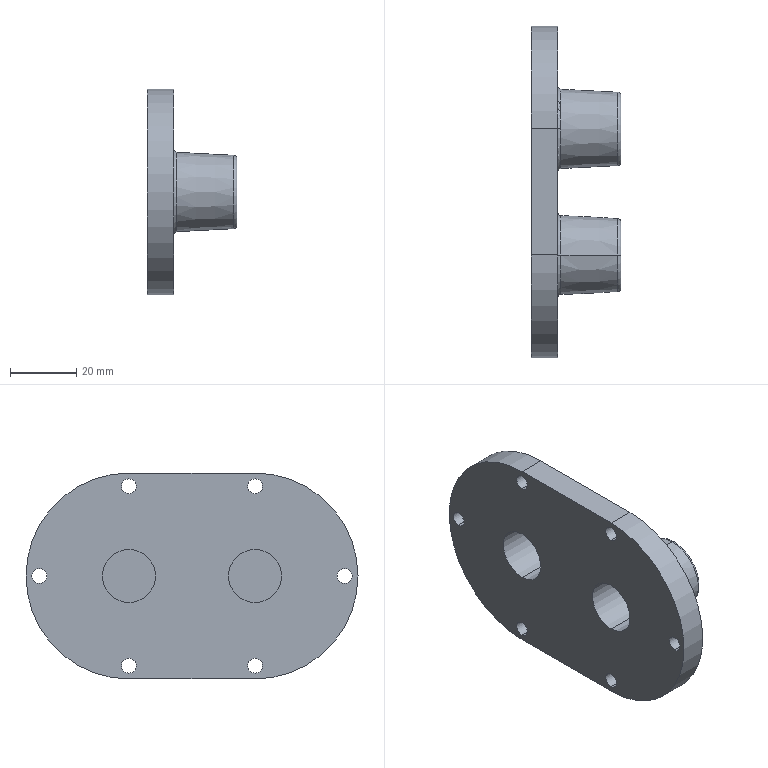Part | SolidWorks | features HoleWzd 2, Revolution 2, Chamfer 1, Extrusion 1, Fillet 1 | 1 solid | 50 faces | box 27 x 100 x 62 mm | volume 48310 mm3 | cylinder 18 | cone 16 | torus 8 | plane 8 | commonest cylinder face diameters 4.5 x12 16 x4 62 x2
STEP:
#1=CARTESIAN_POINT('',(8.948,-19.,11.946));
#2=VERTEX_POINT('',#1);
#3=CARTESIAN_POINT('',(8.948,-19.,-11.946));
#4=VERTEX_POINT('',#3);
#5=CARTESIAN_POINT('',(8.948,-19.,0.));
#6=DIRECTION('',(1.,0.,0.));
#7=DIRECTION('',(0.,0.,1.));
#8=AXIS2_PLACEMENT_3D('',#5,#6,#7);
#9=CIRCLE('',#8,11.946);
#10=EDGE_CURVE('',#2,#4,#9,.T.);
#11=ORIENTED_EDGE('',*,*,#10,.F.);
#12=CARTESIAN_POINT('',(8.,-19.,12.945));
#13=VERTEX_POINT('',#12);
#14=CARTESIAN_POINT('',(9.,-19.,12.945));
#15=DIRECTION('',(0.,1.,0.));
#16=DIRECTION('',(0.,0.,1.));
#17=AXIS2_PLACEMENT_3D('',#14,#15,#16);
#18=CIRCLE('',#17,1.);
#19=EDGE_CURVE('',#2,#13,#18,.T.);
#20=ORIENTED_EDGE('',*,*,#19,.T.);
#21=CARTESIAN_POINT('',(8.,-19.,-12.945));
#22=VERTEX_POINT('',#21);
#23=CARTESIAN_POINT('',(8.,-19.,0.));
#24=DIRECTION('',(-1.,0.,0.));
#25=DIRECTION('',(0.,0.,-1.));
#26=AXIS2_PLACEMENT_3D('',#23,#24,#25);
#27=CIRCLE('',#26,12.945);
#28=EDGE_CURVE('',#22,#13,#27,.T.);
#29=ORIENTED_EDGE('',*,*,#28,.F.);
#30=CARTESIAN_POINT('',(9.,-19.,-12.945));
#31=DIRECTION('',(0.,-1.,0.));
#32=DIRECTION('',(0.,0.,-1.));
#33=AXIS2_PLACEMENT_3D('',#30,#31,#32);
#34=CIRCLE('',#33,1.);
#35=EDGE_CURVE('',#4,#22,#34,.T.);
#36=ORIENTED_EDGE('',*,*,#35,.F.);
#37=EDGE_LOOP('',(#11,#20,#29,#36));
#38=FACE_OUTER_BOUND('',#37,.T.);
#39=CARTESIAN_POINT('',(9.,-19.,0.));
#40=DIRECTION('',(1.,0.,0.));
#41=DIRECTION('',(0.,0.,-1.));
#42=AXIS2_PLACEMENT_3D('',#39,#40,#41);
#43=TOROIDAL_SURFACE('',#42,12.945,1.);
#44=ADVANCED_FACE('',(#38),#43,.F.);
#45=CARTESIAN_POINT('',(26.052,-19.,11.05));
#46=VERTEX_POINT('',#45);
#47=CARTESIAN_POINT('',(26.052,-19.,-11.05));
#48=VERTEX_POINT('',#47);
#49=CARTESIAN_POINT('',(26.052,-19.,0.));
#50=DIRECTION('',(-1.,0.,0.));
#51=DIRECTION('',(0.,0.,-1.));
#52=AXIS2_PLACEMENT_3D('',#49,#50,#51);
#53=CIRCLE('',#52,11.05);
#54=EDGE_CURVE('',#46,#48,#53,.T.);
#55=ORIENTED_EDGE('',*,*,#54,.F.);
#56=CARTESIAN_POINT('',(27.,-19.,10.051));
#57=VERTEX_POINT('',#56);
#58=CARTESIAN_POINT('',(26.,-19.,10.051));
#59=DIRECTION('',(0.,1.,0.));
#60=DIRECTION('',(0.,0.,1.));
#61=AXIS2_PLACEMENT_3D('',#58,#59,#60);
#62=CIRCLE('',#61,1.);
#63=EDGE_CURVE('',#46,#57,#62,.T.);
#64=ORIENTED_EDGE('',*,*,#63,.T.);
#65=CARTESIAN_POINT('',(27.,-19.,-10.051));
#66=VERTEX_POINT('',#65);
#67=CARTESIAN_POINT('',(27.,-19.,0.));
#68=DIRECTION('',(1.,0.,0.));
#69=DIRECTION('',(0.,0.,-1.));
#70=AXIS2_PLACEMENT_3D('',#67,#68,#69);
#71=CIRCLE('',#70,10.051);
#72=EDGE_CURVE('',#66,#57,#71,.T.);
#73=ORIENTED_EDGE('',*,*,#72,.F.);
#74=CARTESIAN_POINT('',(26.,-19.,-10.051));
#75=DIRECTION('',(0.,-1.,0.));
#76=DIRECTION('',(0.,0.,-1.));
#77=AXIS2_PLACEMENT_3D('',#74,#75,#76);
#78=CIRCLE('',#77,1.);
#79=EDGE_CURVE('',#48,#66,#78,.T.);
#80=ORIENTED_EDGE('',*,*,#79,.F.);
#81=EDGE_LOOP('',(#55,#64,#73,#80));
#82=FACE_OUTER_BOUND('',#81,.T.);
#83=CARTESIAN_POINT('',(26.,-19.,0.));
#84=DIRECTION('',(1.,0.,0.));
#85=DIRECTION('',(0.,0.,-1.));
#86=AXIS2_PLACEMENT_3D('',#83,#84,#85);
#87=TOROIDAL_SURFACE('',#86,10.051,1.);
#88=ADVANCED_FACE('',(#82),#87,.T.);
#89=CARTESIAN_POINT('',(8.948,19.,11.946));
#90=VERTEX_POINT('',#89);
#91=CARTESIAN_POINT('',(8.948,7.054,0.));
#92=VERTEX_POINT('',#91);
#93=CARTESIAN_POINT('',(8.948,19.,0.));
#94=DIRECTION('',(1.,0.,0.));
#95=DIRECTION('',(0.,-1.,0.));
#96=AXIS2_PLACEMENT_3D('',#93,#94,#95);
#97=CIRCLE('',#96,11.946);
#98=EDGE_CURVE('',#90,#92,#97,.T.);
#99=ORIENTED_EDGE('',*,*,#98,.F.);
#100=CARTESIAN_POINT('',(8.,19.,12.945));
#101=VERTEX_POINT('',#100);
#102=CARTESIAN_POINT('',(9.,19.,12.945));
#103=DIRECTION('',(0.,1.,0.));
#104=DIRECTION('',(0.,0.,1.));
#105=AXIS2_PLACEMENT_3D('',#102,#103,#104);
#106=CIRCLE('',#105,1.);
#107=EDGE_CURVE('',#90,#101,#106,.T.);
#108=ORIENTED_EDGE('',*,*,#107,.T.);
#109=CARTESIAN_POINT('',(8.,19.,-12.945));
#110=VERTEX_POINT('',#109);
#111=CARTESIAN_POINT('',(8.,19.,0.));
#112=DIRECTION('',(-1.,0.,0.));
#113=DIRECTION('',(0.,0.,-1.));
#114=AXIS2_PLACEMENT_3D('',#111,#112,#113);
#115=CIRCLE('',#114,12.945);
#116=EDGE_CURVE('',#110,#101,#115,.T.);
#117=ORIENTED_EDGE('',*,*,#116,.F.);
#118=CARTESIAN_POINT('',(8.948,19.,-11.946));
#119=VERTEX_POINT('',#118);
#120=CARTESIAN_POINT('',(9.,19.,-12.945));
#121=DIRECTION('',(0.,-1.,0.));
#122=DIRECTION('',(0.,0.,-1.));
#123=AXIS2_PLACEMENT_3D('',#120,#121,#122);
#124=CIRCLE('',#123,1.);
#125=EDGE_CURVE('',#119,#110,#124,.T.);
#126=ORIENTED_EDGE('',*,*,#125,.F.);
#127=CARTESIAN_POINT('',(8.948,19.,0.));
#128=DIRECTION('',(1.,0.,0.));
#129=DIRECTION('',(0.,-1.,0.));
#130=AXIS2_PLACEMENT_3D('',#127,#128,#129);
#131=CIRCLE('',#130,11.946);
#132=EDGE_CURVE('',#92,#119,#131,.T.);
#133=ORIENTED_EDGE('',*,*,#132,.F.);
#134=EDGE_LOOP('',(#99,#108,#117,#126,#133));
#135=FACE_OUTER_BOUND('',#134,.T.);
#136=CARTESIAN_POINT('',(9.,19.,0.));
#137=DIRECTION('',(1.,0.,0.));
#138=DIRECTION('',(0.,0.,-1.));
#139=AXIS2_PLACEMENT_3D('',#136,#137,#138);
#140=TOROIDAL_SURFACE('',#139,12.945,1.);
#141=ADVANCED_FACE('',(#135),#140,.F.);
#142=CARTESIAN_POINT('',(26.052,7.95,0.));
#143=VERTEX_POINT('',#142);
#144=CARTESIAN_POINT('',(26.052,30.05,0.));
#145=VERTEX_POINT('',#144);
#146=CARTESIAN_POINT('',(26.052,19.,0.));
#147=DIRECTION('',(-1.,0.,0.));
#148=DIRECTION('',(0.,1.,0.));
#149=AXIS2_PLACEMENT_3D('',#146,#147,#148);
#150=CIRCLE('',#149,11.05);
#151=EDGE_CURVE('',#143,#145,#150,.T.);
#152=ORIENTED_EDGE('',*,*,#151,.F.);
#153=CARTESIAN_POINT('',(27.,8.949,0.));
#154=VERTEX_POINT('',#153);
#155=CARTESIAN_POINT('',(26.,8.949,0.));
#156=DIRECTION('',(0.,0.,1.));
#157=DIRECTION('',(0.,-1.,0.));
#158=AXIS2_PLACEMENT_3D('',#155,#156,#157);
#159=CIRCLE('',#158,1.);
#160=EDGE_CURVE('',#143,#154,#159,.T.);
#161=ORIENTED_EDGE('',*,*,#160,.T.);
#162=CARTESIAN_POINT('',(27.,29.051,0.));
#163=VERTEX_POINT('',#162);
#164=CARTESIAN_POINT('',(27.,19.,0.));
#165=DIRECTION('',(1.,0.,0.));
#166=DIRECTION('',(0.,1.,0.));
#167=AXIS2_PLACEMENT_3D('',#164,#165,#166);
#168=CIRCLE('',#167,10.051);
#169=EDGE_CURVE('',#163,#154,#168,.T.);
#170=ORIENTED_EDGE('',*,*,#169,.F.);
#171=CARTESIAN_POINT('',(26.,29.051,0.));
#172=DIRECTION('',(0.,0.,-1.));
#173=DIRECTION('',(-1.,0.,0.));
#174=AXIS2_PLACEMENT_3D('',#171,#172,#173);
#175=CIRCLE('',#174,1.);
#176=EDGE_CURVE('',#145,#163,#175,.T.);
#177=ORIENTED_EDGE('',*,*,#176,.F.);
#178=EDGE_LOOP('',(#152,#161,#170,#177));
#179=FACE_OUTER_BOUND('',#178,.T.);
#180=CARTESIAN_POINT('',(26.,19.,0.));
#181=DIRECTION('',(1.,0.,0.));
#182=DIRECTION('',(0.,1.,0.));
#183=AXIS2_PLACEMENT_3D('',#180,#181,#182);
#184=TOROIDAL_SURFACE('',#183,10.051,1.);
#185=ADVANCED_FACE('',(#179),#184,.T.);
#186=CARTESIAN_POINT('',(6.8,19.,-24.75));
#187=VERTEX_POINT('',#186);
#188=CARTESIAN_POINT('',(6.8,19.,-29.25));
#189=VERTEX_POINT('',#188);
#190=CARTESIAN_POINT('',(6.8,19.,-27.));
#191=DIRECTION('',(1.,0.,0.));
#192=DIRECTION('',(0.,0.,-1.));
#193=AXIS2_PLACEMENT_3D('',#190,#191,#192);
#194=CIRCLE('',#193,2.25);
#195=EDGE_CURVE('',#187,#189,#194,.T.);
#196=ORIENTED_EDGE('',*,*,#195,.F.);
#197=CARTESIAN_POINT('',(8.,19.,-23.55));
#198=VERTEX_POINT('',#197);
#199=CARTESIAN_POINT('',(6.8,19.,-24.75));
#200=DIRECTION('',(0.7071,0.,0.7071));
#201=VECTOR('',#200,1000.);
#202=LINE('',#199,#201);
#203=EDGE_CURVE('',#187,#198,#202,.T.);
#204=ORIENTED_EDGE('',*,*,#203,.T.);
#205=CARTESIAN_POINT('',(8.,19.,-30.45));
#206=VERTEX_POINT('',#205);
#207=CARTESIAN_POINT('',(8.,19.,-27.));
#208=DIRECTION('',(-1.,0.,0.));
#209=DIRECTION('',(0.,0.,-1.));
#210=AXIS2_PLACEMENT_3D('',#207,#208,#209);
#211=CIRCLE('',#210,3.45);
#212=EDGE_CURVE('',#206,#198,#211,.T.);
#213=ORIENTED_EDGE('',*,*,#212,.F.);
#214=CARTESIAN_POINT('',(6.8,19.,-29.25));
#215=DIRECTION('',(0.7071,0.,-0.7071));
#216=VECTOR('',#215,1000.);
#217=LINE('',#214,#216);
#218=EDGE_CURVE('',#189,#206,#217,.T.);
#219=ORIENTED_EDGE('',*,*,#218,.F.);
#220=EDGE_LOOP('',(#196,#204,#213,#219));
#221=FACE_OUTER_BOUND('',#220,.T.);
#222=CARTESIAN_POINT('',(6.8,19.,-27.));
#223=DIRECTION('',(1.,0.,0.));
#224=DIRECTION('',(0.,0.,-1.));
#225=AXIS2_PLACEMENT_3D('',#222,#223,#224);
#226=CONICAL_SURFACE('',#225,2.25,0.7854);
#227=ADVANCED_FACE('',(#221),#226,.F.);
#228=CARTESIAN_POINT('',(6.8,-19.,-24.75));
#229=VERTEX_POINT('',#228);
#230=CARTESIAN_POINT('',(6.8,-19.,-29.25));
#231=VERTEX_POINT('',#230);
#232=CARTESIAN_POINT('',(6.8,-19.,-27.));
#233=DIRECTION('',(1.,0.,0.));
#234=DIRECTION('',(0.,0.,-1.));
#235=AXIS2_PLACEMENT_3D('',#232,#233,#234);
#236=CIRCLE('',#235,2.25);
#237=EDGE_CURVE('',#229,#231,#236,.T.);
#238=ORIENTED_EDGE('',*,*,#237,.F.);
#239=CARTESIAN_POINT('',(8.,-19.,-23.55));
#240=VERTEX_POINT('',#239);
#241=CARTESIAN_POINT('',(6.8,-19.,-24.75));
#242=DIRECTION('',(0.7071,0.,0.7071));
#243=VECTOR('',#242,1000.);
#244=LINE('',#241,#243);
#245=EDGE_CURVE('',#229,#240,#244,.T.);
#246=ORIENTED_EDGE('',*,*,#245,.T.);
#247=CARTESIAN_POINT('',(8.,-19.,-30.45));
#248=VERTEX_POINT('',#247);
#249=CARTESIAN_POINT('',(8.,-19.,-27.));
#250=DIRECTION('',(-1.,0.,0.));
#251=DIRECTION('',(0.,0.,-1.));
#252=AXIS2_PLACEMENT_3D('',#249,#250,#251);
#253=CIRCLE('',#252,3.45);
#254=EDGE_CURVE('',#248,#240,#253,.T.);
#255=ORIENTED_EDGE('',*,*,#254,.F.);
#256=CARTESIAN_POINT('',(6.8,-19.,-29.25));
#257=DIRECTION('',(0.7071,0.,-0.7071));
#258=VECTOR('',#257,1000.);
#259=LINE('',#256,#258);
#260=EDGE_CURVE('',#231,#248,#259,.T.);
#261=ORIENTED_EDGE('',*,*,#260,.F.);
#262=EDGE_LOOP('',(#238,#246,#255,#261));
#263=FACE_OUTER_BOUND('',#262,.T.);
#264=CARTESIAN_POINT('',(6.8,-19.,-27.));
#265=DIRECTION('',(1.,0.,0.));
#266=DIRECTION('',(0.,0.,-1.));
#267=AXIS2_PLACEMENT_3D('',#264,#265,#266);
#268=CONICAL_SURFACE('',#267,2.25,0.7854);
#269=ADVANCED_FACE('',(#263),#268,.F.);
#270=CARTESIAN_POINT('',(6.8,19.,29.25));
#271=VERTEX_POINT('',#270);
#272=CARTESIAN_POINT('',(6.8,19.,24.75));
#273=VERTEX_POINT('',#272);
#274=CARTESIAN_POINT('',(6.8,19.,27.));
#275=DIRECTION('',(1.,0.,0.));
#276=DIRECTION('',(0.,0.,-1.));
#277=AXIS2_PLACEMENT_3D('',#274,#275,#276);
#278=CIRCLE('',#277,2.25);
#279=EDGE_CURVE('',#271,#273,#278,.T.);
#280=ORIENTED_EDGE('',*,*,#279,.F.);
#281=CARTESIAN_POINT('',(8.,19.,30.45));
#282=VERTEX_POINT('',#281);
#283=CARTESIAN_POINT('',(6.8,19.,29.25));
#284=DIRECTION('',(0.7071,0.,0.7071));
#285=VECTOR('',#284,1000.);
#286=LINE('',#283,#285);
#287=EDGE_CURVE('',#271,#282,#286,.T.);
#288=ORIENTED_EDGE('',*,*,#287,.T.);
#289=CARTESIAN_POINT('',(8.,19.,23.55));
#290=VERTEX_POINT('',#289);
#291=CARTESIAN_POINT('',(8.,19.,27.));
#292=DIRECTION('',(-1.,0.,0.));
#293=DIRECTION('',(0.,0.,-1.));
#294=AXIS2_PLACEMENT_3D('',#291,#292,#293);
#295=CIRCLE('',#294,3.45);
#296=EDGE_CURVE('',#290,#282,#295,.T.);
#297=ORIENTED_EDGE('',*,*,#296,.F.);
#298=CARTESIAN_POINT('',(6.8,19.,24.75));
#299=DIRECTION('',(0.7071,0.,-0.7071));
#300=VECTOR('',#299,1000.);
#301=LINE('',#298,#300);
#302=EDGE_CURVE('',#273,#290,#301,.T.);
#303=ORIENTED_EDGE('',*,*,#302,.F.);
#304=EDGE_LOOP('',(#280,#288,#297,#303));
#305=FACE_OUTER_BOUND('',#304,.T.);
#306=CARTESIAN_POINT('',(6.8,19.,27.));
#307=DIRECTION('',(1.,0.,0.));
#308=DIRECTION('',(0.,0.,-1.));
#309=AXIS2_PLACEMENT_3D('',#306,#307,#308);
#310=CONICAL_SURFACE('',#309,2.25,0.7854);
#311=ADVANCED_FACE('',(#305),#310,.F.);
#312=CARTESIAN_POINT('',(6.8,46.,2.25));
#313=VERTEX_POINT('',#312);
#314=CARTESIAN_POINT('',(6.8,46.,-2.25));
#315=VERTEX_POINT('',#314);
#316=CARTESIAN_POINT('',(6.8,46.,0.));
#317=DIRECTION('',(1.,0.,0.));
#318=DIRECTION('',(0.,0.,-1.));
#319=AXIS2_PLACEMENT_3D('',#316,#317,#318);
#320=CIRCLE('',#319,2.25);
#321=EDGE_CURVE('',#313,#315,#320,.T.);
#322=ORIENTED_EDGE('',*,*,#321,.F.);
#323=CARTESIAN_POINT('',(8.,46.,3.45));
#324=VERTEX_POINT('',#323);
#325=CARTESIAN_POINT('',(6.8,46.,2.25));
#326=DIRECTION('',(0.7071,0.,0.7071));
#327=VECTOR('',#326,1000.);
#328=LINE('',#325,#327);
#329=EDGE_CURVE('',#313,#324,#328,.T.);
#330=ORIENTED_EDGE('',*,*,#329,.T.);
#331=CARTESIAN_POINT('',(8.,46.,-3.45));
#332=VERTEX_POINT('',#331);
#333=CARTESIAN_POINT('',(8.,46.,0.));
#334=DIRECTION('',(-1.,0.,0.));
#335=DIRECTION('',(0.,0.,-1.));
#336=AXIS2_PLACEMENT_3D('',#333,#334,#335);
#337=CIRCLE('',#336,3.45);
#338=EDGE_CURVE('',#332,#324,#337,.T.);
#339=ORIENTED_EDGE('',*,*,#338,.F.);
#340=CARTESIAN_POINT('',(6.8,46.,-2.25));
#341=DIRECTION('',(0.7071,0.,-0.7071));
#342=VECTOR('',#341,1000.);
#343=LINE('',#340,#342);
#344=EDGE_CURVE('',#315,#332,#343,.T.);
#345=ORIENTED_EDGE('',*,*,#344,.F.);
#346=EDGE_LOOP('',(#322,#330,#339,#345));
#347=FACE_OUTER_BOUND('',#346,.T.);
#348=CARTESIAN_POINT('',(6.8,46.,0.));
#349=DIRECTION('',(1.,0.,0.));
#350=DIRECTION('',(0.,0.,-1.));
#351=AXIS2_PLACEMENT_3D('',#348,#349,#350);
#352=CONICAL_SURFACE('',#351,2.25,0.7854);
#353=ADVANCED_FACE('',(#347),#352,.F.);
#354=CARTESIAN_POINT('',(6.8,-46.,2.25));
#355=VERTEX_POINT('',#354);
#356=CARTESIAN_POINT('',(6.8,-46.,-2.25));
#357=VERTEX_POINT('',#356);
#358=CARTESIAN_POINT('',(6.8,-46.,0.));
#359=DIRECTION('',(1.,0.,0.));
#360=DIRECTION('',(0.,0.,-1.));
#361=AXIS2_PLACEMENT_3D('',#358,#359,#360);
#362=CIRCLE('',#361,2.25);
#363=EDGE_CURVE('',#355,#357,#362,.T.);
#364=ORIENTED_EDGE('',*,*,#363,.F.);
#365=CARTESIAN_POINT('',(8.,-46.,3.45));
#366=VERTEX_POINT('',#365);
#367=CARTESIAN_POINT('',(6.8,-46.,2.25));
#368=DIRECTION('',(0.7071,0.,0.7071));
#369=VECTOR('',#368,1000.);
#370=LINE('',#367,#369);
#371=EDGE_CURVE('',#355,#366,#370,.T.);
#372=ORIENTED_EDGE('',*,*,#371,.T.);
#373=CARTESIAN_POINT('',(8.,-46.,-3.45));
#374=VERTEX_POINT('',#373);
#375=CARTESIAN_POINT('',(8.,-46.,0.));
#376=DIRECTION('',(-1.,0.,0.));
#377=DIRECTION('',(0.,0.,-1.));
#378=AXIS2_PLACEMENT_3D('',#375,#376,#377);
#379=CIRCLE('',#378,3.45);
#380=EDGE_CURVE('',#374,#366,#379,.T.);
#381=ORIENTED_EDGE('',*,*,#380,.F.);
#382=CARTESIAN_POINT('',(6.8,-46.,-2.25));
#383=DIRECTION('',(0.7071,0.,-0.7071));
#384=VECTOR('',#383,1000.);
#385=LINE('',#382,#384);
#386=EDGE_CURVE('',#357,#374,#385,.T.);
#387=ORIENTED_EDGE('',*,*,#386,.F.);
#388=EDGE_LOOP('',(#364,#372,#381,#387));
#389=FACE_OUTER_BOUND('',#388,.T.);
#390=CARTESIAN_POINT('',(6.8,-46.,0.));
#391=DIRECTION('',(1.,0.,0.));
#392=DIRECTION('',(0.,0.,-1.));
#393=AXIS2_PLACEMENT_3D('',#390,#391,#392);
#394=CONICAL_SURFACE('',#393,2.25,0.7854);
#395=ADVANCED_FACE('',(#389),#394,.F.);
#396=CARTESIAN_POINT('',(6.8,-19.,29.25));
#397=VERTEX_POINT('',#396);
#398=CARTESIAN_POINT('',(6.8,-19.,24.75));
#399=VERTEX_POINT('',#398);
#400=CARTESIAN_POINT('',(6.8,-19.,27.));
#401=DIRECTION('',(1.,0.,0.));
#402=DIRECTION('',(0.,0.,-1.));
#403=AXIS2_PLACEMENT_3D('',#400,#401,#402);
#404=CIRCLE('',#403,2.25);
#405=EDGE_CURVE('',#397,#399,#404,.T.);
#406=ORIENTED_EDGE('',*,*,#405,.F.);
#407=CARTESIAN_POINT('',(8.,-19.,30.45));
#408=VERTEX_POINT('',#407);
#409=CARTESIAN_POINT('',(6.8,-19.,29.25));
#410=DIRECTION('',(0.7071,0.,0.7071));
#411=VECTOR('',#410,1000.);
#412=LINE('',#409,#411);
#413=EDGE_CURVE('',#397,#408,#412,.T.);
#414=ORIENTED_EDGE('',*,*,#413,.T.);
#415=CARTESIAN_POINT('',(8.,-19.,23.55));
#416=VERTEX_POINT('',#415);
#417=CARTESIAN_POINT('',(8.,-19.,27.));
#418=DIRECTION('',(-1.,0.,0.));
#419=DIRECTION('',(0.,0.,-1.));
#420=AXIS2_PLACEMENT_3D('',#417,#418,#419);
#421=CIRCLE('',#420,3.45);
#422=EDGE_CURVE('',#416,#408,#421,.T.);
#423=ORIENTED_EDGE('',*,*,#422,.F.);
#424=CARTESIAN_POINT('',(6.8,-19.,24.75));
#425=DIRECTION('',(0.7071,0.,-0.7071));
#426=VECTOR('',#425,1000.);
#427=LINE('',#424,#426);
#428=EDGE_CURVE('',#399,#416,#427,.T.);
#429=ORIENTED_EDGE('',*,*,#428,.F.);
#430=EDGE_LOOP('',(#406,#414,#423,#429));
#431=FACE_OUTER_BOUND('',#430,.T.);
#432=CARTESIAN_POINT('',(6.8,-19.,27.));
#433=DIRECTION('',(1.,0.,0.));
#434=DIRECTION('',(0.,0.,-1.));
#435=AXIS2_PLACEMENT_3D('',#432,#433,#434);
#436=CONICAL_SURFACE('',#435,2.25,0.7854);
#437=ADVANCED_FACE('',(#431),#436,.F.);
#438=CARTESIAN_POINT('',(0.,46.,2.25));
#439=VERTEX_POINT('',#438);
#440=CARTESIAN_POINT('',(0.,46.,-2.25));
#441=VERTEX_POINT('',#440);
#442=CARTESIAN_POINT('',(0.,46.,0.));
#443=DIRECTION('',(1.,0.,0.));
#444=DIRECTION('',(0.,0.,-1.));
#445=AXIS2_PLACEMENT_3D('',#442,#443,#444);
#446=CIRCLE('',#445,2.25);
#447=EDGE_CURVE('',#439,#441,#446,.T.);
#448=ORIENTED_EDGE('',*,*,#447,.F.);
#449=CARTESIAN_POINT('',(8.,46.,2.25));
#450=DIRECTION('',(1.,0.,0.));
#451=VECTOR('',#450,1000.);
#452=LINE('',#449,#451);
#453=EDGE_CURVE('',#439,#313,#452,.T.);
#454=ORIENTED_EDGE('',*,*,#453,.T.);
#455=ORIENTED_EDGE('',*,*,#321,.T.);
#456=CARTESIAN_POINT('',(8.,46.,-2.25));
#457=DIRECTION('',(1.,0.,0.));
#458=VECTOR('',#457,1000.);
#459=LINE('',#456,#458);
#460=EDGE_CURVE('',#441,#315,#459,.T.);
#461=ORIENTED_EDGE('',*,*,#460,.F.);
#462=EDGE_LOOP('',(#448,#454,#455,#461));
#463=FACE_OUTER_BOUND('',#462,.T.);
#464=CARTESIAN_POINT('',(8.,46.,0.));
#465=DIRECTION('',(1.,0.,0.));
#466=DIRECTION('',(0.,0.,-1.));
#467=AXIS2_PLACEMENT_3D('',#464,#465,#466);
#468=CYLINDRICAL_SURFACE('',#467,2.25);
#469=ADVANCED_FACE('',(#463),#468,.F.);
#470=CARTESIAN_POINT('',(0.,19.,29.25));
#471=VERTEX_POINT('',#470);
#472=CARTESIAN_POINT('',(0.,19.,24.75));
#473=VERTEX_POINT('',#472);
#474=CARTESIAN_POINT('',(0.,19.,27.));
#475=DIRECTION('',(1.,0.,0.));
#476=DIRECTION('',(0.,0.,-1.));
#477=AXIS2_PLACEMENT_3D('',#474,#475,#476);
#478=CIRCLE('',#477,2.25);
#479=EDGE_CURVE('',#471,#473,#478,.T.);
#480=ORIENTED_EDGE('',*,*,#479,.F.);
#481=CARTESIAN_POINT('',(8.,19.,29.25));
#482=DIRECTION('',(1.,0.,0.));
#483=VECTOR('',#482,1000.);
#484=LINE('',#481,#483);
#485=EDGE_CURVE('',#471,#271,#484,.T.);
#486=ORIENTED_EDGE('',*,*,#485,.T.);
#487=ORIENTED_EDGE('',*,*,#279,.T.);
#488=CARTESIAN_POINT('',(8.,19.,24.75));
#489=DIRECTION('',(1.,0.,0.));
#490=VECTOR('',#489,1000.);
#491=LINE('',#488,#490);
#492=EDGE_CURVE('',#473,#273,#491,.T.);
#493=ORIENTED_EDGE('',*,*,#492,.F.);
#494=EDGE_LOOP('',(#480,#486,#487,#493));
#495=FACE_OUTER_BOUND('',#494,.T.);
#496=CARTESIAN_POINT('',(8.,19.,27.));
#497=DIRECTION('',(1.,0.,0.));
#498=DIRECTION('',(0.,0.,-1.));
#499=AXIS2_PLACEMENT_3D('',#496,#497,#498);
#500=CYLINDRICAL_SURFACE('',#499,2.25);
#501=ADVANCED_FACE('',(#495),#500,.F.);
#502=CARTESIAN_POINT('',(0.,19.,-24.75));
#503=VERTEX_POINT('',#502);
#504=CARTESIAN_POINT('',(0.,19.,-29.25));
#505=VERTEX_POINT('',#504);
#506=CARTESIAN_POINT('',(0.,19.,-27.));
#507=DIRECTION('',(1.,0.,0.));
#508=DIRECTION('',(0.,0.,-1.));
#509=AXIS2_PLACEMENT_3D('',#506,#507,#508);
#510=CIRCLE('',#509,2.25);
#511=EDGE_CURVE('',#503,#505,#510,.T.);
#512=ORIENTED_EDGE('',*,*,#511,.F.);
#513=CARTESIAN_POINT('',(8.,19.,-24.75));
#514=DIRECTION('',(1.,0.,0.));
#515=VECTOR('',#514,1000.);
#516=LINE('',#513,#515);
#517=EDGE_CURVE('',#503,#187,#516,.T.);
#518=ORIENTED_EDGE('',*,*,#517,.T.);
#519=ORIENTED_EDGE('',*,*,#195,.T.);
#520=CARTESIAN_POINT('',(8.,19.,-29.25));
#521=DIRECTION('',(1.,0.,0.));
#522=VECTOR('',#521,1000.);
#523=LINE('',#520,#522);
#524=EDGE_CURVE('',#505,#189,#523,.T.);
#525=ORIENTED_EDGE('',*,*,#524,.F.);
#526=EDGE_LOOP('',(#512,#518,#519,#525));
#527=FACE_OUTER_BOUND('',#526,.T.);
#528=CARTESIAN_POINT('',(8.,19.,-27.));
#529=DIRECTION('',(1.,0.,0.));
#530=DIRECTION('',(0.,0.,-1.));
#531=AXIS2_PLACEMENT_3D('',#528,#529,#530);
#532=CYLINDRICAL_SURFACE('',#531,2.25);
#533=ADVANCED_FACE('',(#527),#532,.F.);
#534=CARTESIAN_POINT('',(0.,-19.,29.25));
#535=VERTEX_POINT('',#534);
#536=CARTESIAN_POINT('',(0.,-19.,24.75));
#537=VERTEX_POINT('',#536);
#538=CARTESIAN_POINT('',(0.,-19.,27.));
#539=DIRECTION('',(1.,0.,0.));
#540=DIRECTION('',(0.,0.,-1.));
#541=AXIS2_PLACEMENT_3D('',#538,#539,#540);
#542=CIRCLE('',#541,2.25);
#543=EDGE_CURVE('',#535,#537,#542,.T.);
#544=ORIENTED_EDGE('',*,*,#543,.F.);
#545=CARTESIAN_POINT('',(8.,-19.,29.25));
#546=DIRECTION('',(1.,0.,0.));
#547=VECTOR('',#546,1000.);
#548=LINE('',#545,#547);
#549=EDGE_CURVE('',#535,#397,#548,.T.);
#550=ORIENTED_EDGE('',*,*,#549,.T.);
#551=ORIENTED_EDGE('',*,*,#405,.T.);
#552=CARTESIAN_POINT('',(8.,-19.,24.75));
#553=DIRECTION('',(1.,0.,0.));
#554=VECTOR('',#553,1000.);
#555=LINE('',#552,#554);
#556=EDGE_CURVE('',#537,#399,#555,.T.);
#557=ORIENTED_EDGE('',*,*,#556,.F.);
#558=EDGE_LOOP('',(#544,#550,#551,#557));
#559=FACE_OUTER_BOUND('',#558,.T.);
#560=CARTESIAN_POINT('',(8.,-19.,27.));
#561=DIRECTION('',(1.,0.,0.));
#562=DIRECTION('',(0.,0.,-1.));
#563=AXIS2_PLACEMENT_3D('',#560,#561,#562);
#564=CYLINDRICAL_SURFACE('',#563,2.25);
#565=ADVANCED_FACE('',(#559),#564,.F.);
#566=CARTESIAN_POINT('',(0.,-19.,-24.75));
#567=VERTEX_POINT('',#566);
#568=CARTESIAN_POINT('',(0.,-19.,-29.25));
#569=VERTEX_POINT('',#568);
#570=CARTESIAN_POINT('',(0.,-19.,-27.));
#571=DIRECTION('',(1.,0.,0.));
#572=DIRECTION('',(0.,0.,-1.));
#573=AXIS2_PLACEMENT_3D('',#570,#571,#572);
#574=CIRCLE('',#573,2.25);
#575=EDGE_CURVE('',#567,#569,#574,.T.);
#576=ORIENTED_EDGE('',*,*,#575,.F.);
#577=CARTESIAN_POINT('',(8.,-19.,-24.75));
#578=DIRECTION('',(1.,0.,0.));
#579=VECTOR('',#578,1000.);
#580=LINE('',#577,#579);
#581=EDGE_CURVE('',#567,#229,#580,.T.);
#582=ORIENTED_EDGE('',*,*,#581,.T.);
#583=ORIENTED_EDGE('',*,*,#237,.T.);
#584=CARTESIAN_POINT('',(8.,-19.,-29.25));
#585=DIRECTION('',(1.,0.,0.));
#586=VECTOR('',#585,1000.);
#587=LINE('',#584,#586);
#588=EDGE_CURVE('',#569,#231,#587,.T.);
#589=ORIENTED_EDGE('',*,*,#588,.F.);
#590=EDGE_LOOP('',(#576,#582,#583,#589));
#591=FACE_OUTER_BOUND('',#590,.T.);
#592=CARTESIAN_POINT('',(8.,-19.,-27.));
#593=DIRECTION('',(1.,0.,0.));
#594=DIRECTION('',(0.,0.,-1.));
#595=AXIS2_PLACEMENT_3D('',#592,#593,#594);
#596=CYLINDRICAL_SURFACE('',#595,2.25);
#597=ADVANCED_FACE('',(#591),#596,.F.);
#598=CARTESIAN_POINT('',(0.,-46.,2.25));
#599=VERTEX_POINT('',#598);
#600=CARTESIAN_POINT('',(0.,-46.,-2.25));
#601=VERTEX_POINT('',#600);
#602=CARTESIAN_POINT('',(0.,-46.,0.));
#603=DIRECTION('',(1.,0.,0.));
#604=DIRECTION('',(0.,0.,-1.));
#605=AXIS2_PLACEMENT_3D('',#602,#603,#604);
#606=CIRCLE('',#605,2.25);
#607=EDGE_CURVE('',#599,#601,#606,.T.);
#608=ORIENTED_EDGE('',*,*,#607,.F.);
#609=CARTESIAN_POINT('',(8.,-46.,2.25));
#610=DIRECTION('',(1.,0.,0.));
#611=VECTOR('',#610,1000.);
#612=LINE('',#609,#611);
#613=EDGE_CURVE('',#599,#355,#612,.T.);
#614=ORIENTED_EDGE('',*,*,#613,.T.);
#615=ORIENTED_EDGE('',*,*,#363,.T.);
#616=CARTESIAN_POINT('',(8.,-46.,-2.25));
#617=DIRECTION('',(1.,0.,0.));
#618=VECTOR('',#617,1000.);
#619=LINE('',#616,#618);
#620=EDGE_CURVE('',#601,#357,#619,.T.);
#621=ORIENTED_EDGE('',*,*,#620,.F.);
#622=EDGE_LOOP('',(#608,#614,#615,#621));
#623=FACE_OUTER_BOUND('',#622,.T.);
#624=CARTESIAN_POINT('',(8.,-46.,0.));
#625=DIRECTION('',(1.,0.,0.));
#626=DIRECTION('',(0.,0.,-1.));
#627=AXIS2_PLACEMENT_3D('',#624,#625,#626);
#628=CYLINDRICAL_SURFACE('',#627,2.25);
#629=ADVANCED_FACE('',(#623),#628,.F.);
#630=CARTESIAN_POINT('',(24.,19.,-8.));
#631=VERTEX_POINT('',#630);
#632=CARTESIAN_POINT('',(24.,19.,8.));
#633=VERTEX_POINT('',#632);
#634=CARTESIAN_POINT('',(24.,19.,0.));
#635=DIRECTION('',(-1.,0.,0.));
#636=DIRECTION('',(0.,0.,1.));
#637=AXIS2_PLACEMENT_3D('',#634,#635,#636);
#638=CIRCLE('',#637,8.);
#639=EDGE_CURVE('',#631,#633,#638,.T.);
#640=ORIENTED_EDGE('',*,*,#639,.F.);
#641=CARTESIAN_POINT('',(0.,19.,-8.));
#642=VERTEX_POINT('',#641);
#643=CARTESIAN_POINT('',(0.,19.,-8.));
#644=DIRECTION('',(-1.,0.,0.));
#645=VECTOR('',#644,1000.);
#646=LINE('',#643,#645);
#647=EDGE_CURVE('',#631,#642,#646,.T.);
#648=ORIENTED_EDGE('',*,*,#647,.T.);
#649=CARTESIAN_POINT('',(0.,19.,8.));
#650=VERTEX_POINT('',#649);
#651=CARTESIAN_POINT('',(0.,19.,0.));
#652=DIRECTION('',(-1.,0.,0.));
#653=DIRECTION('',(0.,0.,1.));
#654=AXIS2_PLACEMENT_3D('',#651,#652,#653);
#655=CIRCLE('',#654,8.);
#656=EDGE_CURVE('',#642,#650,#655,.T.);
#657=ORIENTED_EDGE('',*,*,#656,.T.);
#658=CARTESIAN_POINT('',(0.,19.,8.));
#659=DIRECTION('',(-1.,0.,0.));
#660=VECTOR('',#659,1000.);
#661=LINE('',#658,#660);
#662=EDGE_CURVE('',#633,#650,#661,.T.);
#663=ORIENTED_EDGE('',*,*,#662,.F.);
#664=EDGE_LOOP('',(#640,#648,#657,#663));
#665=FACE_OUTER_BOUND('',#664,.T.);
#666=CARTESIAN_POINT('',(0.,19.,0.));
#667=DIRECTION('',(-1.,0.,0.));
#668=DIRECTION('',(0.,0.,1.));
#669=AXIS2_PLACEMENT_3D('',#666,#667,#668);
#670=CYLINDRICAL_SURFACE('',#669,8.);
#671=ADVANCED_FACE('',(#665),#670,.F.);
#672=CARTESIAN_POINT('',(24.,-19.,-8.));
#673=VERTEX_POINT('',#672);
#674=CARTESIAN_POINT('',(24.,-19.,8.));
#675=VERTEX_POINT('',#674);
#676=CARTESIAN_POINT('',(24.,-19.,0.));
#677=DIRECTION('',(-1.,0.,0.));
#678=DIRECTION('',(0.,0.,1.));
#679=AXIS2_PLACEMENT_3D('',#676,#677,#678);
#680=CIRCLE('',#679,8.);
#681=EDGE_CURVE('',#673,#675,#680,.T.);
#682=ORIENTED_EDGE('',*,*,#681,.F.);
#683=CARTESIAN_POINT('',(0.,-19.,-8.));
#684=VERTEX_POINT('',#683);
#685=CARTESIAN_POINT('',(0.,-19.,-8.));
#686=DIRECTION('',(-1.,0.,0.));
#687=VECTOR('',#686,1000.);
#688=LINE('',#685,#687);
#689=EDGE_CURVE('',#673,#684,#688,.T.);
#690=ORIENTED_EDGE('',*,*,#689,.T.);
#691=CARTESIAN_POINT('',(0.,-19.,8.));
#692=VERTEX_POINT('',#691);
#693=CARTESIAN_POINT('',(0.,-19.,0.));
#694=DIRECTION('',(-1.,0.,0.));
#695=DIRECTION('',(0.,0.,1.));
#696=AXIS2_PLACEMENT_3D('',#693,#694,#695);
#697=CIRCLE('',#696,8.);
#698=EDGE_CURVE('',#684,#692,#697,.T.);
#699=ORIENTED_EDGE('',*,*,#698,.T.);
#700=CARTESIAN_POINT('',(0.,-19.,8.));
#701=DIRECTION('',(-1.,0.,0.));
#702=VECTOR('',#701,1000.);
#703=LINE('',#700,#702);
#704=EDGE_CURVE('',#675,#692,#703,.T.);
#705=ORIENTED_EDGE('',*,*,#704,.F.);
#706=EDGE_LOOP('',(#682,#690,#699,#705));
#707=FACE_OUTER_BOUND('',#706,.T.);
#708=CARTESIAN_POINT('',(0.,-19.,0.));
#709=DIRECTION('',(-1.,0.,0.));
#710=DIRECTION('',(0.,0.,1.));
#711=AXIS2_PLACEMENT_3D('',#708,#709,#710);
#712=CYLINDRICAL_SURFACE('',#711,8.);
#713=ADVANCED_FACE('',(#707),#712,.F.);
#714=ORIENTED_EDGE('',*,*,#151,.T.);
#715=CARTESIAN_POINT('',(8.948,30.946,0.));
#716=VERTEX_POINT('',#715);
#717=CARTESIAN_POINT('',(27.,30.,0.));
#718=DIRECTION('',(-0.9986,0.05234,0.));
#719=VECTOR('',#718,1000.);
#720=LINE('',#717,#719);
#721=EDGE_CURVE('',#145,#716,#720,.T.);
#722=ORIENTED_EDGE('',*,*,#721,.T.);
#723=CARTESIAN_POINT('',(8.948,19.,0.));
#724=DIRECTION('',(1.,0.,0.));
#725=DIRECTION('',(0.,-1.,0.));
#726=AXIS2_PLACEMENT_3D('',#723,#724,#725);
#727=CIRCLE('',#726,11.946);
#728=EDGE_CURVE('',#716,#90,#727,.T.);
#729=ORIENTED_EDGE('',*,*,#728,.T.);
#730=ORIENTED_EDGE('',*,*,#98,.T.);
#731=CARTESIAN_POINT('',(27.,8.,0.));
#732=DIRECTION('',(-0.9986,-0.05234,0.));
#733=VECTOR('',#732,1000.);
#734=LINE('',#731,#733);
#735=EDGE_CURVE('',#143,#92,#734,.T.);
#736=ORIENTED_EDGE('',*,*,#735,.F.);
#737=EDGE_LOOP('',(#714,#722,#729,#730,#736));
#738=FACE_OUTER_BOUND('',#737,.T.);
#739=CARTESIAN_POINT('',(27.,19.,0.));
#740=DIRECTION('',(-1.,0.,0.));
#741=DIRECTION('',(0.,-1.,0.));
#742=AXIS2_PLACEMENT_3D('',#739,#740,#741);
#743=CONICAL_SURFACE('',#742,11.,0.05236);
#744=ADVANCED_FACE('',(#738),#743,.T.);
#745=ORIENTED_EDGE('',*,*,#54,.T.);
#746=CARTESIAN_POINT('',(27.,-19.,-11.));
#747=DIRECTION('',(-0.9986,0.,-0.05234));
#748=VECTOR('',#747,1000.);
#749=LINE('',#746,#748);
#750=EDGE_CURVE('',#48,#4,#749,.T.);
#751=ORIENTED_EDGE('',*,*,#750,.T.);
#752=CARTESIAN_POINT('',(8.948,-19.,0.));
#753=DIRECTION('',(1.,0.,0.));
#754=DIRECTION('',(0.,0.,1.));
#755=AXIS2_PLACEMENT_3D('',#752,#753,#754);
#756=CIRCLE('',#755,11.946);
#757=EDGE_CURVE('',#4,#2,#756,.T.);
#758=ORIENTED_EDGE('',*,*,#757,.T.);
#759=CARTESIAN_POINT('',(27.,-19.,11.));
#760=DIRECTION('',(-0.9986,0.,0.05234));
#761=VECTOR('',#760,1000.);
#762=LINE('',#759,#761);
#763=EDGE_CURVE('',#46,#2,#762,.T.);
#764=ORIENTED_EDGE('',*,*,#763,.F.);
#765=EDGE_LOOP('',(#745,#751,#758,#764));
#766=FACE_OUTER_BOUND('',#765,.T.);
#767=CARTESIAN_POINT('',(27.,-19.,0.));
#768=DIRECTION('',(-1.,0.,0.));
#769=DIRECTION('',(0.,0.,1.));
#770=AXIS2_PLACEMENT_3D('',#767,#768,#769);
#771=CONICAL_SURFACE('',#770,11.,0.05236);
#772=ADVANCED_FACE('',(#766),#771,.T.);
#773=CARTESIAN_POINT('',(8.,-19.,31.));
#774=VERTEX_POINT('',#773);
#775=CARTESIAN_POINT('',(8.,-19.,-31.));
#776=VERTEX_POINT('',#775);
#777=CARTESIAN_POINT('',(8.,-19.,0.));
#778=DIRECTION('',(1.,0.,0.));
#779=DIRECTION('',(0.,0.,-1.));
#780=AXIS2_PLACEMENT_3D('',#777,#778,#779);
#781=CIRCLE('',#780,31.);
#782=EDGE_CURVE('',#774,#776,#781,.T.);
#783=ORIENTED_EDGE('',*,*,#782,.F.);
#784=CARTESIAN_POINT('',(0.,-19.,31.));
#785=VERTEX_POINT('',#784);
#786=CARTESIAN_POINT('',(0.,-19.,31.));
#787=DIRECTION('',(1.,0.,0.));
#788=VECTOR('',#787,1000.);
#789=LINE('',#786,#788);
#790=EDGE_CURVE('',#785,#774,#789,.T.);
#791=ORIENTED_EDGE('',*,*,#790,.F.);
#792=CARTESIAN_POINT('',(0.,-19.,-31.));
#793=VERTEX_POINT('',#792);
#794=CARTESIAN_POINT('',(0.,-19.,0.));
#795=DIRECTION('',(1.,0.,0.));
#796=DIRECTION('',(0.,0.,-1.));
#797=AXIS2_PLACEMENT_3D('',#794,#795,#796);
#798=CIRCLE('',#797,31.);
#799=EDGE_CURVE('',#785,#793,#798,.T.);
#800=ORIENTED_EDGE('',*,*,#799,.T.);
#801=CARTESIAN_POINT('',(0.,-19.,-31.));
#802=DIRECTION('',(1.,0.,0.));
#803=VECTOR('',#802,1000.);
#804=LINE('',#801,#803);
#805=EDGE_CURVE('',#793,#776,#804,.T.);
#806=ORIENTED_EDGE('',*,*,#805,.T.);
#807=EDGE_LOOP('',(#783,#791,#800,#806));
#808=FACE_OUTER_BOUND('',#807,.T.);
#809=CARTESIAN_POINT('',(0.,-19.,0.));
#810=DIRECTION('',(1.,0.,0.));
#811=DIRECTION('',(0.,0.,-1.));
#812=AXIS2_PLACEMENT_3D('',#809,#810,#811);
#813=CYLINDRICAL_SURFACE('',#812,31.);
#814=ADVANCED_FACE('',(#808),#813,.T.);
#815=CARTESIAN_POINT('',(8.,19.,31.));
#816=VERTEX_POINT('',#815);
#817=CARTESIAN_POINT('',(8.,19.,31.));
#818=DIRECTION('',(0.,-1.,0.));
#819=VECTOR('',#818,1000.);
#820=LINE('',#817,#819);
#821=EDGE_CURVE('',#816,#774,#820,.T.);
#822=ORIENTED_EDGE('',*,*,#821,.F.);
#823=CARTESIAN_POINT('',(0.,19.,31.));
#824=VERTEX_POINT('',#823);
#825=CARTESIAN_POINT('',(0.,19.,31.));
#826=DIRECTION('',(1.,0.,0.));
#827=VECTOR('',#826,1000.);
#828=LINE('',#825,#827);
#829=EDGE_CURVE('',#824,#816,#828,.T.);
#830=ORIENTED_EDGE('',*,*,#829,.F.);
#831=CARTESIAN_POINT('',(0.,19.,31.));
#832=DIRECTION('',(0.,-1.,0.));
#833=VECTOR('',#832,1000.);
#834=LINE('',#831,#833);
#835=EDGE_CURVE('',#824,#785,#834,.T.);
#836=ORIENTED_EDGE('',*,*,#835,.T.);
#837=ORIENTED_EDGE('',*,*,#790,.T.);
#838=EDGE_LOOP('',(#822,#830,#836,#837));
#839=FACE_OUTER_BOUND('',#838,.T.);
#840=CARTESIAN_POINT('',(0.,19.,31.));
#841=DIRECTION('',(0.,0.,1.));
#842=DIRECTION('',(1.,0.,0.));
#843=AXIS2_PLACEMENT_3D('',#840,#841,#842);
#844=PLANE('',#843);
#845=ADVANCED_FACE('',(#839),#844,.T.);
#846=CARTESIAN_POINT('',(8.,19.,-31.));
#847=VERTEX_POINT('',#846);
#848=CARTESIAN_POINT('',(8.,19.,0.));
#849=DIRECTION('',(1.,0.,0.));
#850=DIRECTION('',(0.,0.,-1.));
#851=AXIS2_PLACEMENT_3D('',#848,#849,#850);
#852=CIRCLE('',#851,31.);
#853=EDGE_CURVE('',#847,#816,#852,.T.);
#854=ORIENTED_EDGE('',*,*,#853,.F.);
#855=CARTESIAN_POINT('',(0.,19.,-31.));
#856=VERTEX_POINT('',#855);
#857=CARTESIAN_POINT('',(0.,19.,-31.));
#858=DIRECTION('',(1.,0.,0.));
#859=VECTOR('',#858,1000.);
#860=LINE('',#857,#859);
#861=EDGE_CURVE('',#856,#847,#860,.T.);
#862=ORIENTED_EDGE('',*,*,#861,.F.);
#863=CARTESIAN_POINT('',(0.,19.,0.));
#864=DIRECTION('',(1.,0.,0.));
#865=DIRECTION('',(0.,0.,-1.));
#866=AXIS2_PLACEMENT_3D('',#863,#864,#865);
#867=CIRCLE('',#866,31.);
#868=EDGE_CURVE('',#856,#824,#867,.T.);
#869=ORIENTED_EDGE('',*,*,#868,.T.);
#870=ORIENTED_EDGE('',*,*,#829,.T.);
#871=EDGE_LOOP('',(#854,#862,#869,#870));
#872=FACE_OUTER_BOUND('',#871,.T.);
#873=CARTESIAN_POINT('',(0.,19.,0.));
#874=DIRECTION('',(1.,0.,0.));
#875=DIRECTION('',(0.,0.,-1.));
#876=AXIS2_PLACEMENT_3D('',#873,#874,#875);
#877=CYLINDRICAL_SURFACE('',#876,31.);
#878=ADVANCED_FACE('',(#872),#877,.T.);
#879=CARTESIAN_POINT('',(8.,-19.,-31.));
#880=DIRECTION('',(0.,1.,0.));
#881=VECTOR('',#880,1000.);
#882=LINE('',#879,#881);
#883=EDGE_CURVE('',#776,#847,#882,.T.);
#884=ORIENTED_EDGE('',*,*,#883,.F.);
#885=ORIENTED_EDGE('',*,*,#805,.F.);
#886=CARTESIAN_POINT('',(0.,-19.,-31.));
#887=DIRECTION('',(0.,1.,0.));
#888=VECTOR('',#887,1000.);
#889=LINE('',#886,#888);
#890=EDGE_CURVE('',#793,#856,#889,.T.);
#891=ORIENTED_EDGE('',*,*,#890,.T.);
#892=ORIENTED_EDGE('',*,*,#861,.T.);
#893=EDGE_LOOP('',(#884,#885,#891,#892));
#894=FACE_OUTER_BOUND('',#893,.T.);
#895=CARTESIAN_POINT('',(0.,-19.,-31.));
#896=DIRECTION('',(0.,0.,-1.));
#897=DIRECTION('',(-1.,0.,0.));
#898=AXIS2_PLACEMENT_3D('',#895,#896,#897);
#899=PLANE('',#898);
#900=ADVANCED_FACE('',(#894),#899,.T.);
#901=CARTESIAN_POINT('',(0.,46.,0.));
#902=DIRECTION('',(1.,0.,0.));
#903=DIRECTION('',(0.,0.,-1.));
#904=AXIS2_PLACEMENT_3D('',#901,#902,#903);
#905=CIRCLE('',#904,2.25);
#906=EDGE_CURVE('',#441,#439,#905,.T.);
#907=ORIENTED_EDGE('',*,*,#906,.T.);
#908=ORIENTED_EDGE('',*,*,#447,.T.);
#909=EDGE_LOOP('',(#907,#908));
#910=FACE_BOUND('',#909,.T.);
#911=CARTESIAN_POINT('',(0.,19.,27.));
#912=DIRECTION('',(1.,0.,0.));
#913=DIRECTION('',(0.,0.,-1.));
#914=AXIS2_PLACEMENT_3D('',#911,#912,#913);
#915=CIRCLE('',#914,2.25);
#916=EDGE_CURVE('',#473,#471,#915,.T.);
#917=ORIENTED_EDGE('',*,*,#916,.T.);
#918=ORIENTED_EDGE('',*,*,#479,.T.);
#919=EDGE_LOOP('',(#917,#918));
#920=FACE_BOUND('',#919,.T.);
#921=CARTESIAN_POINT('',(0.,19.,-27.));
#922=DIRECTION('',(1.,0.,0.));
#923=DIRECTION('',(0.,0.,-1.));
#924=AXIS2_PLACEMENT_3D('',#921,#922,#923);
#925=CIRCLE('',#924,2.25);
#926=EDGE_CURVE('',#505,#503,#925,.T.);
#927=ORIENTED_EDGE('',*,*,#926,.T.);
#928=ORIENTED_EDGE('',*,*,#511,.T.);
#929=EDGE_LOOP('',(#927,#928));
#930=FACE_BOUND('',#929,.T.);
#931=CARTESIAN_POINT('',(0.,-19.,27.));
#932=DIRECTION('',(1.,0.,0.));
#933=DIRECTION('',(0.,0.,-1.));
#934=AXIS2_PLACEMENT_3D('',#931,#932,#933);
#935=CIRCLE('',#934,2.25);
#936=EDGE_CURVE('',#537,#535,#935,.T.);
#937=ORIENTED_EDGE('',*,*,#936,.T.);
#938=ORIENTED_EDGE('',*,*,#543,.T.);
#939=EDGE_LOOP('',(#937,#938));
#940=FACE_BOUND('',#939,.T.);
#941=CARTESIAN_POINT('',(0.,-19.,-27.));
#942=DIRECTION('',(1.,0.,0.));
#943=DIRECTION('',(0.,0.,-1.));
#944=AXIS2_PLACEMENT_3D('',#941,#942,#943);
#945=CIRCLE('',#944,2.25);
#946=EDGE_CURVE('',#569,#567,#945,.T.);
#947=ORIENTED_EDGE('',*,*,#946,.T.);
#948=ORIENTED_EDGE('',*,*,#575,.T.);
#949=EDGE_LOOP('',(#947,#948));
#950=FACE_BOUND('',#949,.T.);
#951=CARTESIAN_POINT('',(0.,-46.,0.));
#952=DIRECTION('',(1.,0.,0.));
#953=DIRECTION('',(0.,0.,-1.));
#954=AXIS2_PLACEMENT_3D('',#951,#952,#953);
#955=CIRCLE('',#954,2.25);
#956=EDGE_CURVE('',#601,#599,#955,.T.);
#957=ORIENTED_EDGE('',*,*,#956,.T.);
#958=ORIENTED_EDGE('',*,*,#607,.T.);
#959=EDGE_LOOP('',(#957,#958));
#960=FACE_BOUND('',#959,.T.);
#961=CARTESIAN_POINT('',(0.,19.,0.));
#962=DIRECTION('',(-1.,0.,0.));
#963=DIRECTION('',(0.,0.,1.));
#964=AXIS2_PLACEMENT_3D('',#961,#962,#963);
#965=CIRCLE('',#964,8.);
#966=EDGE_CURVE('',#650,#642,#965,.T.);
#967=ORIENTED_EDGE('',*,*,#966,.F.);
#968=ORIENTED_EDGE('',*,*,#656,.F.);
#969=EDGE_LOOP('',(#967,#968));
#970=FACE_BOUND('',#969,.T.);
#971=CARTESIAN_POINT('',(0.,-19.,0.));
#972=DIRECTION('',(-1.,0.,0.));
#973=DIRECTION('',(0.,0.,1.));
#974=AXIS2_PLACEMENT_3D('',#971,#972,#973);
#975=CIRCLE('',#974,8.);
#976=EDGE_CURVE('',#692,#684,#975,.T.);
#977=ORIENTED_EDGE('',*,*,#976,.F.);
#978=ORIENTED_EDGE('',*,*,#698,.F.);
#979=EDGE_LOOP('',(#977,#978));
#980=FACE_BOUND('',#979,.T.);
#981=ORIENTED_EDGE('',*,*,#799,.F.);
#982=ORIENTED_EDGE('',*,*,#835,.F.);
#983=ORIENTED_EDGE('',*,*,#868,.F.);
#984=ORIENTED_EDGE('',*,*,#890,.F.);
#985=EDGE_LOOP('',(#981,#982,#983,#984));
#986=FACE_OUTER_BOUND('',#985,.T.);
#987=CARTESIAN_POINT('',(0.,-19.,0.));
#988=DIRECTION('',(1.,0.,0.));
#989=DIRECTION('',(0.,0.,-1.));
#990=AXIS2_PLACEMENT_3D('',#987,#988,#989);
#991=PLANE('',#990);
#992=ADVANCED_FACE('',(#910,#920,#930,#940,#950,#960,#970,#980,#986),#991,.F.);
#993=ORIENTED_EDGE('',*,*,#116,.T.);
#994=CARTESIAN_POINT('',(8.,19.,0.));
#995=DIRECTION('',(-1.,0.,0.));
#996=DIRECTION('',(0.,0.,-1.));
#997=AXIS2_PLACEMENT_3D('',#994,#995,#996);
#998=CIRCLE('',#997,12.945);
#999=EDGE_CURVE('',#101,#110,#998,.T.);
#1000=ORIENTED_EDGE('',*,*,#999,.T.);
#1001=EDGE_LOOP('',(#993,#1000));
#1002=FACE_BOUND('',#1001,.T.);
#1003=ORIENTED_EDGE('',*,*,#28,.T.);
#1004=CARTESIAN_POINT('',(8.,-19.,0.));
#1005=DIRECTION('',(-1.,0.,0.));
#1006=DIRECTION('',(0.,0.,-1.));
#1007=AXIS2_PLACEMENT_3D('',#1004,#1005,#1006);
#1008=CIRCLE('',#1007,12.945);
#1009=EDGE_CURVE('',#13,#22,#1008,.T.);
#1010=ORIENTED_EDGE('',*,*,#1009,.T.);
#1011=EDGE_LOOP('',(#1003,#1010));
#1012=FACE_BOUND('',#1011,.T.);
#1013=ORIENTED_EDGE('',*,*,#422,.T.);
#1014=CARTESIAN_POINT('',(8.,-19.,27.));
#1015=DIRECTION('',(-1.,0.,0.));
#1016=DIRECTION('',(0.,0.,-1.));
#1017=AXIS2_PLACEMENT_3D('',#1014,#1015,#1016);
#1018=CIRCLE('',#1017,3.45);
#1019=EDGE_CURVE('',#408,#416,#1018,.T.);
#1020=ORIENTED_EDGE('',*,*,#1019,.T.);
#1021=EDGE_LOOP('',(#1013,#1020));
#1022=FACE_BOUND('',#1021,.T.);
#1023=ORIENTED_EDGE('',*,*,#380,.T.);
#1024=CARTESIAN_POINT('',(8.,-46.,0.));
#1025=DIRECTION('',(-1.,0.,0.));
#1026=DIRECTION('',(0.,0.,-1.));
#1027=AXIS2_PLACEMENT_3D('',#1024,#1025,#1026);
#1028=CIRCLE('',#1027,3.45);
#1029=EDGE_CURVE('',#366,#374,#1028,.T.);
#1030=ORIENTED_EDGE('',*,*,#1029,.T.);
#1031=EDGE_LOOP('',(#1023,#1030));
#1032=FACE_BOUND('',#1031,.T.);
#1033=ORIENTED_EDGE('',*,*,#338,.T.);
#1034=CARTESIAN_POINT('',(8.,46.,0.));
#1035=DIRECTION('',(-1.,0.,0.));
#1036=DIRECTION('',(0.,0.,-1.));
#1037=AXIS2_PLACEMENT_3D('',#1034,#1035,#1036);
#1038=CIRCLE('',#1037,3.45);
#1039=EDGE_CURVE('',#324,#332,#1038,.T.);
#1040=ORIENTED_EDGE('',*,*,#1039,.T.);
#1041=EDGE_LOOP('',(#1033,#1040));
#1042=FACE_BOUND('',#1041,.T.);
#1043=ORIENTED_EDGE('',*,*,#296,.T.);
#1044=CARTESIAN_POINT('',(8.,19.,27.));
#1045=DIRECTION('',(-1.,0.,0.));
#1046=DIRECTION('',(0.,0.,-1.));
#1047=AXIS2_PLACEMENT_3D('',#1044,#1045,#1046);
#1048=CIRCLE('',#1047,3.45);
#1049=EDGE_CURVE('',#282,#290,#1048,.T.);
#1050=ORIENTED_EDGE('',*,*,#1049,.T.);
#1051=EDGE_LOOP('',(#1043,#1050));
#1052=FACE_BOUND('',#1051,.T.);
#1053=ORIENTED_EDGE('',*,*,#254,.T.);
#1054=CARTESIAN_POINT('',(8.,-19.,-27.));
#1055=DIRECTION('',(-1.,0.,0.));
#1056=DIRECTION('',(0.,0.,-1.));
#1057=AXIS2_PLACEMENT_3D('',#1054,#1055,#1056);
#1058=CIRCLE('',#1057,3.45);
#1059=EDGE_CURVE('',#240,#248,#1058,.T.);
#1060=ORIENTED_EDGE('',*,*,#1059,.T.);
#1061=EDGE_LOOP('',(#1053,#1060));
#1062=FACE_BOUND('',#1061,.T.);
#1063=ORIENTED_EDGE('',*,*,#212,.T.);
#1064=CARTESIAN_POINT('',(8.,19.,-27.));
#1065=DIRECTION('',(-1.,0.,0.));
#1066=DIRECTION('',(0.,0.,-1.));
#1067=AXIS2_PLACEMENT_3D('',#1064,#1065,#1066);
#1068=CIRCLE('',#1067,3.45);
#1069=EDGE_CURVE('',#198,#206,#1068,.T.);
#1070=ORIENTED_EDGE('',*,*,#1069,.T.);
#1071=EDGE_LOOP('',(#1063,#1070));
#1072=FACE_BOUND('',#1071,.T.);
#1073=ORIENTED_EDGE('',*,*,#782,.T.);
#1074=ORIENTED_EDGE('',*,*,#883,.T.);
#1075=ORIENTED_EDGE('',*,*,#853,.T.);
#1076=ORIENTED_EDGE('',*,*,#821,.T.);
#1077=EDGE_LOOP('',(#1073,#1074,#1075,#1076));
#1078=FACE_OUTER_BOUND('',#1077,.T.);
#1079=CARTESIAN_POINT('',(8.,-19.,0.));
#1080=DIRECTION('',(1.,0.,0.));
#1081=DIRECTION('',(0.,0.,-1.));
#1082=AXIS2_PLACEMENT_3D('',#1079,#1080,#1081);
#1083=PLANE('',#1082);
#1084=ADVANCED_FACE('',(#1002,#1012,#1022,#1032,#1042,#1052,#1062,#1072,#1078),#1083,.T.);
#1085=ORIENTED_EDGE('',*,*,#750,.F.);
#1086=CARTESIAN_POINT('',(26.052,-19.,0.));
#1087=DIRECTION('',(-1.,0.,0.));
#1088=DIRECTION('',(0.,0.,-1.));
#1089=AXIS2_PLACEMENT_3D('',#1086,#1087,#1088);
#1090=CIRCLE('',#1089,11.05);
#1091=EDGE_CURVE('',#48,#46,#1090,.T.);
#1092=ORIENTED_EDGE('',*,*,#1091,.T.);
#1093=ORIENTED_EDGE('',*,*,#763,.T.);
#1094=ORIENTED_EDGE('',*,*,#10,.T.);
#1095=EDGE_LOOP('',(#1085,#1092,#1093,#1094));
#1096=FACE_OUTER_BOUND('',#1095,.T.);
#1097=CARTESIAN_POINT('',(27.,-19.,0.));
#1098=DIRECTION('',(-1.,0.,0.));
#1099=DIRECTION('',(0.,0.,1.));
#1100=AXIS2_PLACEMENT_3D('',#1097,#1098,#1099);
#1101=CONICAL_SURFACE('',#1100,11.,0.05236);
#1102=ADVANCED_FACE('',(#1096),#1101,.T.);
#1103=ORIENTED_EDGE('',*,*,#72,.T.);
#1104=CARTESIAN_POINT('',(27.,-19.,0.));
#1105=DIRECTION('',(1.,0.,0.));
#1106=DIRECTION('',(0.,0.,-1.));
#1107=AXIS2_PLACEMENT_3D('',#1104,#1105,#1106);
#1108=CIRCLE('',#1107,10.051);
#1109=EDGE_CURVE('',#57,#66,#1108,.T.);
#1110=ORIENTED_EDGE('',*,*,#1109,.T.);
#1111=EDGE_LOOP('',(#1103,#1110));
#1112=FACE_OUTER_BOUND('',#1111,.T.);
#1113=CARTESIAN_POINT('',(27.,-19.,0.));
#1114=DIRECTION('',(1.,0.,0.));
#1115=DIRECTION('',(0.,0.,-1.));
#1116=AXIS2_PLACEMENT_3D('',#1113,#1114,#1115);
#1117=PLANE('',#1116);
#1118=ADVANCED_FACE('',(#1112),#1117,.T.);
#1119=ORIENTED_EDGE('',*,*,#721,.F.);
#1120=CARTESIAN_POINT('',(26.052,19.,0.));
#1121=DIRECTION('',(-1.,0.,0.));
#1122=DIRECTION('',(0.,1.,0.));
#1123=AXIS2_PLACEMENT_3D('',#1120,#1121,#1122);
#1124=CIRCLE('',#1123,11.05);
#1125=EDGE_CURVE('',#145,#143,#1124,.T.);
#1126=ORIENTED_EDGE('',*,*,#1125,.T.);
#1127=ORIENTED_EDGE('',*,*,#735,.T.);
#1128=ORIENTED_EDGE('',*,*,#132,.T.);
#1129=CARTESIAN_POINT('',(8.948,19.,0.));
#1130=DIRECTION('',(1.,0.,0.));
#1131=DIRECTION('',(0.,-1.,0.));
#1132=AXIS2_PLACEMENT_3D('',#1129,#1130,#1131);
#1133=CIRCLE('',#1132,11.946);
#1134=EDGE_CURVE('',#119,#716,#1133,.T.);
#1135=ORIENTED_EDGE('',*,*,#1134,.T.);
#1136=EDGE_LOOP('',(#1119,#1126,#1127,#1128,#1135));
#1137=FACE_OUTER_BOUND('',#1136,.T.);
#1138=CARTESIAN_POINT('',(27.,19.,0.));
#1139=DIRECTION('',(-1.,0.,0.));
#1140=DIRECTION('',(0.,-1.,0.));
#1141=AXIS2_PLACEMENT_3D('',#1138,#1139,#1140);
#1142=CONICAL_SURFACE('',#1141,11.,0.05236);
#1143=ADVANCED_FACE('',(#1137),#1142,.T.);
#1144=ORIENTED_EDGE('',*,*,#169,.T.);
#1145=CARTESIAN_POINT('',(27.,19.,0.));
#1146=DIRECTION('',(1.,0.,0.));
#1147=DIRECTION('',(0.,1.,0.));
#1148=AXIS2_PLACEMENT_3D('',#1145,#1146,#1147);
#1149=CIRCLE('',#1148,10.051);
#1150=EDGE_CURVE('',#154,#163,#1149,.T.);
#1151=ORIENTED_EDGE('',*,*,#1150,.T.);
#1152=EDGE_LOOP('',(#1144,#1151));
#1153=FACE_OUTER_BOUND('',#1152,.T.);
#1154=CARTESIAN_POINT('',(27.,19.,0.));
#1155=DIRECTION('',(1.,0.,0.));
#1156=DIRECTION('',(0.,1.,0.));
#1157=AXIS2_PLACEMENT_3D('',#1154,#1155,#1156);
#1158=PLANE('',#1157);
#1159=ADVANCED_FACE('',(#1153),#1158,.T.);
#1160=CARTESIAN_POINT('',(24.,-19.,0.));
#1161=DIRECTION('',(-1.,0.,0.));
#1162=DIRECTION('',(0.,0.,1.));
#1163=AXIS2_PLACEMENT_3D('',#1160,#1161,#1162);
#1164=CIRCLE('',#1163,8.);
#1165=EDGE_CURVE('',#675,#673,#1164,.T.);
#1166=ORIENTED_EDGE('',*,*,#1165,.T.);
#1167=ORIENTED_EDGE('',*,*,#681,.T.);
#1168=EDGE_LOOP('',(#1166,#1167));
#1169=FACE_OUTER_BOUND('',#1168,.T.);
#1170=CARTESIAN_POINT('',(24.,-19.,0.));
#1171=DIRECTION('',(1.,0.,0.));
#1172=DIRECTION('',(0.,0.,-1.));
#1173=AXIS2_PLACEMENT_3D('',#1170,#1171,#1172);
#1174=PLANE('',#1173);
#1175=ADVANCED_FACE('',(#1169),#1174,.F.);
#1176=ORIENTED_EDGE('',*,*,#689,.F.);
#1177=ORIENTED_EDGE('',*,*,#1165,.F.);
#1178=ORIENTED_EDGE('',*,*,#704,.T.);
#1179=ORIENTED_EDGE('',*,*,#976,.T.);
#1180=EDGE_LOOP('',(#1176,#1177,#1178,#1179));
#1181=FACE_OUTER_BOUND('',#1180,.T.);
#1182=CARTESIAN_POINT('',(0.,-19.,0.));
#1183=DIRECTION('',(-1.,0.,0.));
#1184=DIRECTION('',(0.,0.,1.));
#1185=AXIS2_PLACEMENT_3D('',#1182,#1183,#1184);
#1186=CYLINDRICAL_SURFACE('',#1185,8.);
#1187=ADVANCED_FACE('',(#1181),#1186,.F.);
#1188=CARTESIAN_POINT('',(24.,19.,0.));
#1189=DIRECTION('',(-1.,0.,0.));
#1190=DIRECTION('',(0.,0.,1.));
#1191=AXIS2_PLACEMENT_3D('',#1188,#1189,#1190);
#1192=CIRCLE('',#1191,8.);
#1193=EDGE_CURVE('',#633,#631,#1192,.T.);
#1194=ORIENTED_EDGE('',*,*,#1193,.T.);
#1195=ORIENTED_EDGE('',*,*,#639,.T.);
#1196=EDGE_LOOP('',(#1194,#1195));
#1197=FACE_OUTER_BOUND('',#1196,.T.);
#1198=CARTESIAN_POINT('',(24.,19.,0.));
#1199=DIRECTION('',(1.,0.,0.));
#1200=DIRECTION('',(0.,0.,-1.));
#1201=AXIS2_PLACEMENT_3D('',#1198,#1199,#1200);
#1202=PLANE('',#1201);
#1203=ADVANCED_FACE('',(#1197),#1202,.F.);
#1204=ORIENTED_EDGE('',*,*,#647,.F.);
#1205=ORIENTED_EDGE('',*,*,#1193,.F.);
#1206=ORIENTED_EDGE('',*,*,#662,.T.);
#1207=ORIENTED_EDGE('',*,*,#966,.T.);
#1208=EDGE_LOOP('',(#1204,#1205,#1206,#1207));
#1209=FACE_OUTER_BOUND('',#1208,.T.);
#1210=CARTESIAN_POINT('',(0.,19.,0.));
#1211=DIRECTION('',(-1.,0.,0.));
#1212=DIRECTION('',(0.,0.,1.));
#1213=AXIS2_PLACEMENT_3D('',#1210,#1211,#1212);
#1214=CYLINDRICAL_SURFACE('',#1213,8.);
#1215=ADVANCED_FACE('',(#1209),#1214,.F.);
#1216=ORIENTED_EDGE('',*,*,#613,.F.);
#1217=ORIENTED_EDGE('',*,*,#956,.F.);
#1218=ORIENTED_EDGE('',*,*,#620,.T.);
#1219=CARTESIAN_POINT('',(6.8,-46.,0.));
#1220=DIRECTION('',(1.,0.,0.));
#1221=DIRECTION('',(0.,0.,-1.));
#1222=AXIS2_PLACEMENT_3D('',#1219,#1220,#1221);
#1223=CIRCLE('',#1222,2.25);
#1224=EDGE_CURVE('',#357,#355,#1223,.T.);
#1225=ORIENTED_EDGE('',*,*,#1224,.T.);
#1226=EDGE_LOOP('',(#1216,#1217,#1218,#1225));
#1227=FACE_OUTER_BOUND('',#1226,.T.);
#1228=CARTESIAN_POINT('',(8.,-46.,0.));
#1229=DIRECTION('',(1.,0.,0.));
#1230=DIRECTION('',(0.,0.,-1.));
#1231=AXIS2_PLACEMENT_3D('',#1228,#1229,#1230);
#1232=CYLINDRICAL_SURFACE('',#1231,2.25);
#1233=ADVANCED_FACE('',(#1227),#1232,.F.);
#1234=ORIENTED_EDGE('',*,*,#581,.F.);
#1235=ORIENTED_EDGE('',*,*,#946,.F.);
#1236=ORIENTED_EDGE('',*,*,#588,.T.);
#1237=CARTESIAN_POINT('',(6.8,-19.,-27.));
#1238=DIRECTION('',(1.,0.,0.));
#1239=DIRECTION('',(0.,0.,-1.));
#1240=AXIS2_PLACEMENT_3D('',#1237,#1238,#1239);
#1241=CIRCLE('',#1240,2.25);
#1242=EDGE_CURVE('',#231,#229,#1241,.T.);
#1243=ORIENTED_EDGE('',*,*,#1242,.T.);
#1244=EDGE_LOOP('',(#1234,#1235,#1236,#1243));
#1245=FACE_OUTER_BOUND('',#1244,.T.);
#1246=CARTESIAN_POINT('',(8.,-19.,-27.));
#1247=DIRECTION('',(1.,0.,0.));
#1248=DIRECTION('',(0.,0.,-1.));
#1249=AXIS2_PLACEMENT_3D('',#1246,#1247,#1248);
#1250=CYLINDRICAL_SURFACE('',#1249,2.25);
#1251=ADVANCED_FACE('',(#1245),#1250,.F.);
#1252=ORIENTED_EDGE('',*,*,#549,.F.);
#1253=ORIENTED_EDGE('',*,*,#936,.F.);
#1254=ORIENTED_EDGE('',*,*,#556,.T.);
#1255=CARTESIAN_POINT('',(6.8,-19.,27.));
#1256=DIRECTION('',(1.,0.,0.));
#1257=DIRECTION('',(0.,0.,-1.));
#1258=AXIS2_PLACEMENT_3D('',#1255,#1256,#1257);
#1259=CIRCLE('',#1258,2.25);
#1260=EDGE_CURVE('',#399,#397,#1259,.T.);
#1261=ORIENTED_EDGE('',*,*,#1260,.T.);
#1262=EDGE_LOOP('',(#1252,#1253,#1254,#1261));
#1263=FACE_OUTER_BOUND('',#1262,.T.);
#1264=CARTESIAN_POINT('',(8.,-19.,27.));
#1265=DIRECTION('',(1.,0.,0.));
#1266=DIRECTION('',(0.,0.,-1.));
#1267=AXIS2_PLACEMENT_3D('',#1264,#1265,#1266);
#1268=CYLINDRICAL_SURFACE('',#1267,2.25);
#1269=ADVANCED_FACE('',(#1263),#1268,.F.);
#1270=ORIENTED_EDGE('',*,*,#517,.F.);
#1271=ORIENTED_EDGE('',*,*,#926,.F.);
#1272=ORIENTED_EDGE('',*,*,#524,.T.);
#1273=CARTESIAN_POINT('',(6.8,19.,-27.));
#1274=DIRECTION('',(1.,0.,0.));
#1275=DIRECTION('',(0.,0.,-1.));
#1276=AXIS2_PLACEMENT_3D('',#1273,#1274,#1275);
#1277=CIRCLE('',#1276,2.25);
#1278=EDGE_CURVE('',#189,#187,#1277,.T.);
#1279=ORIENTED_EDGE('',*,*,#1278,.T.);
#1280=EDGE_LOOP('',(#1270,#1271,#1272,#1279));
#1281=FACE_OUTER_BOUND('',#1280,.T.);
#1282=CARTESIAN_POINT('',(8.,19.,-27.));
#1283=DIRECTION('',(1.,0.,0.));
#1284=DIRECTION('',(0.,0.,-1.));
#1285=AXIS2_PLACEMENT_3D('',#1282,#1283,#1284);
#1286=CYLINDRICAL_SURFACE('',#1285,2.25);
#1287=ADVANCED_FACE('',(#1281),#1286,.F.);
#1288=ORIENTED_EDGE('',*,*,#485,.F.);
#1289=ORIENTED_EDGE('',*,*,#916,.F.);
#1290=ORIENTED_EDGE('',*,*,#492,.T.);
#1291=CARTESIAN_POINT('',(6.8,19.,27.));
#1292=DIRECTION('',(1.,0.,0.));
#1293=DIRECTION('',(0.,0.,-1.));
#1294=AXIS2_PLACEMENT_3D('',#1291,#1292,#1293);
#1295=CIRCLE('',#1294,2.25);
#1296=EDGE_CURVE('',#273,#271,#1295,.T.);
#1297=ORIENTED_EDGE('',*,*,#1296,.T.);
#1298=EDGE_LOOP('',(#1288,#1289,#1290,#1297));
#1299=FACE_OUTER_BOUND('',#1298,.T.);
#1300=CARTESIAN_POINT('',(8.,19.,27.));
#1301=DIRECTION('',(1.,0.,0.));
#1302=DIRECTION('',(0.,0.,-1.));
#1303=AXIS2_PLACEMENT_3D('',#1300,#1301,#1302);
#1304=CYLINDRICAL_SURFACE('',#1303,2.25);
#1305=ADVANCED_FACE('',(#1299),#1304,.F.);
#1306=ORIENTED_EDGE('',*,*,#453,.F.);
#1307=ORIENTED_EDGE('',*,*,#906,.F.);
#1308=ORIENTED_EDGE('',*,*,#460,.T.);
#1309=CARTESIAN_POINT('',(6.8,46.,0.));
#1310=DIRECTION('',(1.,0.,0.));
#1311=DIRECTION('',(0.,0.,-1.));
#1312=AXIS2_PLACEMENT_3D('',#1309,#1310,#1311);
#1313=CIRCLE('',#1312,2.25);
#1314=EDGE_CURVE('',#315,#313,#1313,.T.);
#1315=ORIENTED_EDGE('',*,*,#1314,.T.);
#1316=EDGE_LOOP('',(#1306,#1307,#1308,#1315));
#1317=FACE_OUTER_BOUND('',#1316,.T.);
#1318=CARTESIAN_POINT('',(8.,46.,0.));
#1319=DIRECTION('',(1.,0.,0.));
#1320=DIRECTION('',(0.,0.,-1.));
#1321=AXIS2_PLACEMENT_3D('',#1318,#1319,#1320);
#1322=CYLINDRICAL_SURFACE('',#1321,2.25);
#1323=ADVANCED_FACE('',(#1317),#1322,.F.);
#1324=ORIENTED_EDGE('',*,*,#413,.F.);
#1325=ORIENTED_EDGE('',*,*,#1260,.F.);
#1326=ORIENTED_EDGE('',*,*,#428,.T.);
#1327=ORIENTED_EDGE('',*,*,#1019,.F.);
#1328=EDGE_LOOP('',(#1324,#1325,#1326,#1327));
#1329=FACE_OUTER_BOUND('',#1328,.T.);
#1330=CARTESIAN_POINT('',(6.8,-19.,27.));
#1331=DIRECTION('',(1.,0.,0.));
#1332=DIRECTION('',(0.,0.,-1.));
#1333=AXIS2_PLACEMENT_3D('',#1330,#1331,#1332);
#1334=CONICAL_SURFACE('',#1333,2.25,0.7854);
#1335=ADVANCED_FACE('',(#1329),#1334,.F.);
#1336=ORIENTED_EDGE('',*,*,#371,.F.);
#1337=ORIENTED_EDGE('',*,*,#1224,.F.);
#1338=ORIENTED_EDGE('',*,*,#386,.T.);
#1339=ORIENTED_EDGE('',*,*,#1029,.F.);
#1340=EDGE_LOOP('',(#1336,#1337,#1338,#1339));
#1341=FACE_OUTER_BOUND('',#1340,.T.);
#1342=CARTESIAN_POINT('',(6.8,-46.,0.));
#1343=DIRECTION('',(1.,0.,0.));
#1344=DIRECTION('',(0.,0.,-1.));
#1345=AXIS2_PLACEMENT_3D('',#1342,#1343,#1344);
#1346=CONICAL_SURFACE('',#1345,2.25,0.7854);
#1347=ADVANCED_FACE('',(#1341),#1346,.F.);
#1348=ORIENTED_EDGE('',*,*,#329,.F.);
#1349=ORIENTED_EDGE('',*,*,#1314,.F.);
#1350=ORIENTED_EDGE('',*,*,#344,.T.);
#1351=ORIENTED_EDGE('',*,*,#1039,.F.);
#1352=EDGE_LOOP('',(#1348,#1349,#1350,#1351));
#1353=FACE_OUTER_BOUND('',#1352,.T.);
#1354=CARTESIAN_POINT('',(6.8,46.,0.));
#1355=DIRECTION('',(1.,0.,0.));
#1356=DIRECTION('',(0.,0.,-1.));
#1357=AXIS2_PLACEMENT_3D('',#1354,#1355,#1356);
#1358=CONICAL_SURFACE('',#1357,2.25,0.7854);
#1359=ADVANCED_FACE('',(#1353),#1358,.F.);
#1360=ORIENTED_EDGE('',*,*,#287,.F.);
#1361=ORIENTED_EDGE('',*,*,#1296,.F.);
#1362=ORIENTED_EDGE('',*,*,#302,.T.);
#1363=ORIENTED_EDGE('',*,*,#1049,.F.);
#1364=EDGE_LOOP('',(#1360,#1361,#1362,#1363));
#1365=FACE_OUTER_BOUND('',#1364,.T.);
#1366=CARTESIAN_POINT('',(6.8,19.,27.));
#1367=DIRECTION('',(1.,0.,0.));
#1368=DIRECTION('',(0.,0.,-1.));
#1369=AXIS2_PLACEMENT_3D('',#1366,#1367,#1368);
#1370=CONICAL_SURFACE('',#1369,2.25,0.7854);
#1371=ADVANCED_FACE('',(#1365),#1370,.F.);
#1372=ORIENTED_EDGE('',*,*,#245,.F.);
#1373=ORIENTED_EDGE('',*,*,#1242,.F.);
#1374=ORIENTED_EDGE('',*,*,#260,.T.);
#1375=ORIENTED_EDGE('',*,*,#1059,.F.);
#1376=EDGE_LOOP('',(#1372,#1373,#1374,#1375));
#1377=FACE_OUTER_BOUND('',#1376,.T.);
#1378=CARTESIAN_POINT('',(6.8,-19.,-27.));
#1379=DIRECTION('',(1.,0.,0.));
#1380=DIRECTION('',(0.,0.,-1.));
#1381=AXIS2_PLACEMENT_3D('',#1378,#1379,#1380);
#1382=CONICAL_SURFACE('',#1381,2.25,0.7854);
#1383=ADVANCED_FACE('',(#1377),#1382,.F.);
#1384=ORIENTED_EDGE('',*,*,#203,.F.);
#1385=ORIENTED_EDGE('',*,*,#1278,.F.);
#1386=ORIENTED_EDGE('',*,*,#218,.T.);
#1387=ORIENTED_EDGE('',*,*,#1069,.F.);
#1388=EDGE_LOOP('',(#1384,#1385,#1386,#1387));
#1389=FACE_OUTER_BOUND('',#1388,.T.);
#1390=CARTESIAN_POINT('',(6.8,19.,-27.));
#1391=DIRECTION('',(1.,0.,0.));
#1392=DIRECTION('',(0.,0.,-1.));
#1393=AXIS2_PLACEMENT_3D('',#1390,#1391,#1392);
#1394=CONICAL_SURFACE('',#1393,2.25,0.7854);
#1395=ADVANCED_FACE('',(#1389),#1394,.F.);
#1396=ORIENTED_EDGE('',*,*,#160,.F.);
#1397=ORIENTED_EDGE('',*,*,#1125,.F.);
#1398=ORIENTED_EDGE('',*,*,#176,.T.);
#1399=ORIENTED_EDGE('',*,*,#1150,.F.);
#1400=EDGE_LOOP('',(#1396,#1397,#1398,#1399));
#1401=FACE_OUTER_BOUND('',#1400,.T.);
#1402=CARTESIAN_POINT('',(26.,19.,0.));
#1403=DIRECTION('',(1.,0.,0.));
#1404=DIRECTION('',(0.,1.,0.));
#1405=AXIS2_PLACEMENT_3D('',#1402,#1403,#1404);
#1406=TOROIDAL_SURFACE('',#1405,10.051,1.);
#1407=ADVANCED_FACE('',(#1401),#1406,.T.);
#1408=ORIENTED_EDGE('',*,*,#107,.F.);
#1409=ORIENTED_EDGE('',*,*,#728,.F.);
#1410=ORIENTED_EDGE('',*,*,#1134,.F.);
#1411=ORIENTED_EDGE('',*,*,#125,.T.);
#1412=ORIENTED_EDGE('',*,*,#999,.F.);
#1413=EDGE_LOOP('',(#1408,#1409,#1410,#1411,#1412));
#1414=FACE_OUTER_BOUND('',#1413,.T.);
#1415=CARTESIAN_POINT('',(9.,19.,0.));
#1416=DIRECTION('',(1.,0.,0.));
#1417=DIRECTION('',(0.,0.,-1.));
#1418=AXIS2_PLACEMENT_3D('',#1415,#1416,#1417);
#1419=TOROIDAL_SURFACE('',#1418,12.945,1.);
#1420=ADVANCED_FACE('',(#1414),#1419,.F.);
#1421=ORIENTED_EDGE('',*,*,#63,.F.);
#1422=ORIENTED_EDGE('',*,*,#1091,.F.);
#1423=ORIENTED_EDGE('',*,*,#79,.T.);
#1424=ORIENTED_EDGE('',*,*,#1109,.F.);
#1425=EDGE_LOOP('',(#1421,#1422,#1423,#1424));
#1426=FACE_OUTER_BOUND('',#1425,.T.);
#1427=CARTESIAN_POINT('',(26.,-19.,0.));
#1428=DIRECTION('',(1.,0.,0.));
#1429=DIRECTION('',(0.,0.,-1.));
#1430=AXIS2_PLACEMENT_3D('',#1427,#1428,#1429);
#1431=TOROIDAL_SURFACE('',#1430,10.051,1.);
#1432=ADVANCED_FACE('',(#1426),#1431,.T.);
#1433=ORIENTED_EDGE('',*,*,#19,.F.);
#1434=ORIENTED_EDGE('',*,*,#757,.F.);
#1435=ORIENTED_EDGE('',*,*,#35,.T.);
#1436=ORIENTED_EDGE('',*,*,#1009,.F.);
#1437=EDGE_LOOP('',(#1433,#1434,#1435,#1436));
#1438=FACE_OUTER_BOUND('',#1437,.T.);
#1439=CARTESIAN_POINT('',(9.,-19.,0.));
#1440=DIRECTION('',(1.,0.,0.));
#1441=DIRECTION('',(0.,0.,-1.));
#1442=AXIS2_PLACEMENT_3D('',#1439,#1440,#1441);
#1443=TOROIDAL_SURFACE('',#1442,12.945,1.);
#1444=ADVANCED_FACE('',(#1438),#1443,.F.);
#1445=CLOSED_SHELL('',(#44,#88,#141,#185,#227,#269,#311,#353,#395,#437,#469,#501,#533,#565,#597,#629,#671,#713,#744,#772,#814,#845,#878,#900,#992,#1084,#1102,#1118,#1143,#1159,#1175,#1187,#1203,#1215,#1233,#1251,#1269,#1287,#1305,#1323,#1335,#1347,#1359,#1371,#1383,#1395,#1407,#1420,#1432,#1444));
#1446=MANIFOLD_SOLID_BREP('',#1445);
#1447=CARTESIAN_POINT('',(0.,0.,0.));
#1448=DIRECTION('',(0.,0.,1.));
#1449=DIRECTION('',(1.,0.,0.));
#1450=AXIS2_PLACEMENT_3D('',#1447,#1448,#1449);
#1451=(LENGTH_UNIT()NAMED_UNIT(*)SI_UNIT(.MILLI.,.METRE.));
#1452=UNCERTAINTY_MEASURE_WITH_UNIT(LENGTH_MEASURE(0.00001),#1451,'','');
#1453=(NAMED_UNIT(*)PLANE_ANGLE_UNIT()SI_UNIT($,.RADIAN.));
#1454=(NAMED_UNIT(*)SI_UNIT($,.STERADIAN.)SOLID_ANGLE_UNIT());
#1455=(GEOMETRIC_REPRESENTATION_CONTEXT(3)GLOBAL_UNCERTAINTY_ASSIGNED_CONTEXT((#1452))GLOBAL_UNIT_ASSIGNED_CONTEXT((#1451,#1453,#1454))REPRESENTATION_CONTEXT('',''));
#1456=ADVANCED_BREP_SHAPE_REPRESENTATION('',(#1446,#1450),#1455);